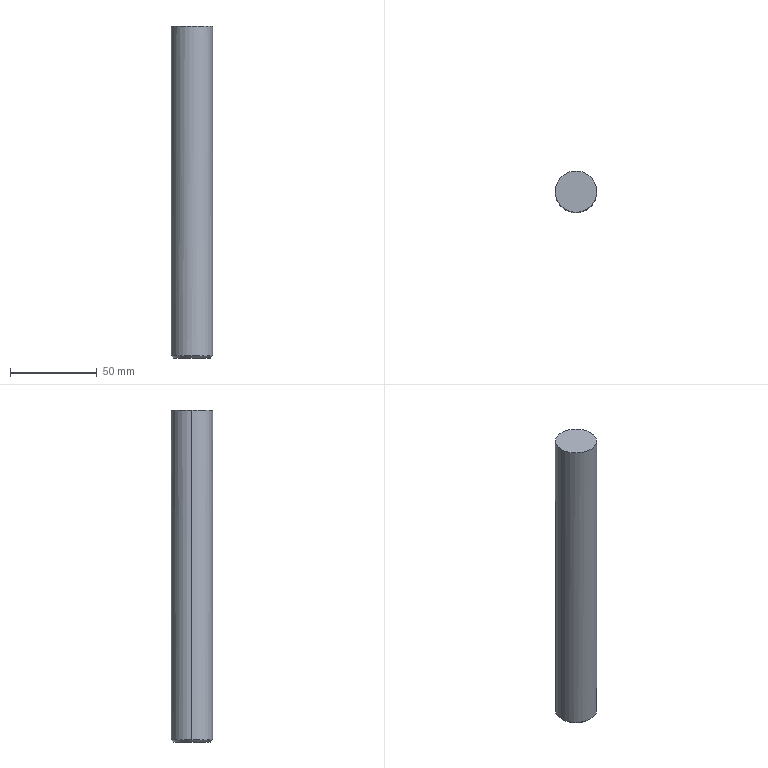Part | SolidWorks | features BaseBody 1 | 1 solid | 13 faces | box 23.8 x 23.8 x 191 mm | volume 54008 mm3 | plane 6 | cylinder 5 | cone 2 | commonest cylinder face diameters 14 x3 23.8 x2
STEP:
#1=CARTESIAN_POINT('',(0.,11.9,-103.8));
#2=VERTEX_POINT('',#1);
#3=CARTESIAN_POINT('',(-11.9,0.,-103.8));
#4=VERTEX_POINT('',#3);
#5=CARTESIAN_POINT('',(0.,0.,-103.8));
#6=DIRECTION('',(0.,0.,1.));
#7=DIRECTION('',(1.,0.,0.));
#8=AXIS2_PLACEMENT_3D('',#5,#6,#7);
#9=CIRCLE('',#8,11.9);
#10=EDGE_CURVE('',#2,#4,#9,.T.);
#11=ORIENTED_EDGE('',*,*,#10,.T.);
#12=CARTESIAN_POINT('',(-11.9,0.,86.));
#13=VERTEX_POINT('',#12);
#14=CARTESIAN_POINT('',(-11.9,0.,90.));
#15=DIRECTION('',(0.,0.,1.));
#16=VECTOR('',#15,1000.);
#17=LINE('',#14,#16);
#18=EDGE_CURVE('',#4,#13,#17,.T.);
#19=ORIENTED_EDGE('',*,*,#18,.T.);
#20=CARTESIAN_POINT('',(11.9,0.,86.));
#21=VERTEX_POINT('',#20);
#22=CARTESIAN_POINT('',(0.,0.,86.));
#23=DIRECTION('',(0.,0.,-1.));
#24=DIRECTION('',(1.,0.,0.));
#25=AXIS2_PLACEMENT_3D('',#22,#23,#24);
#26=CIRCLE('',#25,11.9);
#27=EDGE_CURVE('',#13,#21,#26,.T.);
#28=ORIENTED_EDGE('',*,*,#27,.T.);
#29=CARTESIAN_POINT('',(11.9,0.,-103.8));
#30=VERTEX_POINT('',#29);
#31=CARTESIAN_POINT('',(11.9,0.,90.));
#32=DIRECTION('',(0.,0.,1.));
#33=VECTOR('',#32,1000.);
#34=LINE('',#31,#33);
#35=EDGE_CURVE('',#30,#21,#34,.T.);
#36=ORIENTED_EDGE('',*,*,#35,.F.);
#37=CARTESIAN_POINT('',(0.,0.,-103.8));
#38=DIRECTION('',(0.,0.,1.));
#39=DIRECTION('',(1.,0.,0.));
#40=AXIS2_PLACEMENT_3D('',#37,#38,#39);
#41=CIRCLE('',#40,11.9);
#42=EDGE_CURVE('',#30,#2,#41,.T.);
#43=ORIENTED_EDGE('',*,*,#42,.T.);
#44=EDGE_LOOP('',(#11,#19,#28,#36,#43));
#45=FACE_OUTER_BOUND('',#44,.T.);
#46=CARTESIAN_POINT('',(0.,0.,90.));
#47=DIRECTION('',(0.,0.,1.));
#48=DIRECTION('',(1.,0.,0.));
#49=AXIS2_PLACEMENT_3D('',#46,#47,#48);
#50=CYLINDRICAL_SURFACE('',#49,11.9);
#51=ADVANCED_FACE('',(#45),#50,.T.);
#52=CARTESIAN_POINT('',(0.,-10.7,-105.));
#53=VERTEX_POINT('',#52);
#54=CARTESIAN_POINT('',(0.,10.7,-105.));
#55=VERTEX_POINT('',#54);
#56=CARTESIAN_POINT('',(0.,0.,-105.));
#57=DIRECTION('',(0.,0.,1.));
#58=DIRECTION('',(0.,-1.,0.));
#59=AXIS2_PLACEMENT_3D('',#56,#57,#58);
#60=CIRCLE('',#59,10.7);
#61=EDGE_CURVE('',#53,#55,#60,.T.);
#62=ORIENTED_EDGE('',*,*,#61,.T.);
#63=CARTESIAN_POINT('',(0.,11.9,-103.8));
#64=DIRECTION('',(0.,0.7071,0.7071));
#65=VECTOR('',#64,1000.);
#66=LINE('',#63,#65);
#67=EDGE_CURVE('',#55,#2,#66,.T.);
#68=ORIENTED_EDGE('',*,*,#67,.T.);
#69=ORIENTED_EDGE('',*,*,#42,.F.);
#70=CARTESIAN_POINT('',(0.,-11.9,-103.8));
#71=VERTEX_POINT('',#70);
#72=CARTESIAN_POINT('',(0.,0.,-103.8));
#73=DIRECTION('',(0.,0.,1.));
#74=DIRECTION('',(1.,0.,0.));
#75=AXIS2_PLACEMENT_3D('',#72,#73,#74);
#76=CIRCLE('',#75,11.9);
#77=EDGE_CURVE('',#71,#30,#76,.T.);
#78=ORIENTED_EDGE('',*,*,#77,.F.);
#79=CARTESIAN_POINT('',(0.,-11.9,-103.8));
#80=DIRECTION('',(0.,-0.7071,0.7071));
#81=VECTOR('',#80,1000.);
#82=LINE('',#79,#81);
#83=EDGE_CURVE('',#53,#71,#82,.T.);
#84=ORIENTED_EDGE('',*,*,#83,.F.);
#85=EDGE_LOOP('',(#62,#68,#69,#78,#84));
#86=FACE_OUTER_BOUND('',#85,.T.);
#87=CARTESIAN_POINT('',(0.,0.,-103.8));
#88=DIRECTION('',(0.,0.,1.));
#89=DIRECTION('',(0.,-1.,0.));
#90=AXIS2_PLACEMENT_3D('',#87,#88,#89);
#91=CONICAL_SURFACE('',#90,11.9,0.7854);
#92=ADVANCED_FACE('',(#86),#91,.T.);
#93=CARTESIAN_POINT('',(7.,0.,-105.));
#94=VERTEX_POINT('',#93);
#95=CARTESIAN_POINT('',(-7.,0.,-105.));
#96=VERTEX_POINT('',#95);
#97=CARTESIAN_POINT('',(0.,0.,-105.));
#98=DIRECTION('',(0.,0.,-1.));
#99=DIRECTION('',(1.,0.,0.));
#100=AXIS2_PLACEMENT_3D('',#97,#98,#99);
#101=CIRCLE('',#100,7.);
#102=EDGE_CURVE('',#94,#96,#101,.T.);
#103=ORIENTED_EDGE('',*,*,#102,.T.);
#104=CARTESIAN_POINT('',(-7.,0.,81.));
#105=VERTEX_POINT('',#104);
#106=CARTESIAN_POINT('',(-7.,0.,90.));
#107=DIRECTION('',(0.,0.,1.));
#108=VECTOR('',#107,1000.);
#109=LINE('',#106,#108);
#110=EDGE_CURVE('',#96,#105,#109,.T.);
#111=ORIENTED_EDGE('',*,*,#110,.T.);
#112=CARTESIAN_POINT('',(7.,0.,81.));
#113=VERTEX_POINT('',#112);
#114=CARTESIAN_POINT('',(0.,0.,81.));
#115=DIRECTION('',(0.,0.,-1.));
#116=DIRECTION('',(1.,0.,0.));
#117=AXIS2_PLACEMENT_3D('',#114,#115,#116);
#118=CIRCLE('',#117,7.);
#119=EDGE_CURVE('',#113,#105,#118,.T.);
#120=ORIENTED_EDGE('',*,*,#119,.F.);
#121=CARTESIAN_POINT('',(7.,0.,90.));
#122=DIRECTION('',(0.,0.,1.));
#123=VECTOR('',#122,1000.);
#124=LINE('',#121,#123);
#125=EDGE_CURVE('',#94,#113,#124,.T.);
#126=ORIENTED_EDGE('',*,*,#125,.F.);
#127=EDGE_LOOP('',(#103,#111,#120,#126));
#128=FACE_OUTER_BOUND('',#127,.T.);
#129=CARTESIAN_POINT('',(0.,0.,90.));
#130=DIRECTION('',(0.,0.,1.));
#131=DIRECTION('',(1.,0.,0.));
#132=AXIS2_PLACEMENT_3D('',#129,#130,#131);
#133=CYLINDRICAL_SURFACE('',#132,7.);
#134=ADVANCED_FACE('',(#128),#133,.F.);
#135=CARTESIAN_POINT('',(2.5,6.538,-105.));
#136=VERTEX_POINT('',#135);
#137=CARTESIAN_POINT('',(0.,0.,-105.));
#138=DIRECTION('',(0.,0.,-1.));
#139=DIRECTION('',(1.,0.,0.));
#140=AXIS2_PLACEMENT_3D('',#137,#138,#139);
#141=CIRCLE('',#140,7.);
#142=EDGE_CURVE('',#136,#94,#141,.T.);
#143=ORIENTED_EDGE('',*,*,#142,.T.);
#144=ORIENTED_EDGE('',*,*,#125,.T.);
#145=CARTESIAN_POINT('',(2.5,6.538,81.));
#146=VERTEX_POINT('',#145);
#147=CARTESIAN_POINT('',(0.,0.,81.));
#148=DIRECTION('',(0.,0.,-1.));
#149=DIRECTION('',(1.,0.,0.));
#150=AXIS2_PLACEMENT_3D('',#147,#148,#149);
#151=CIRCLE('',#150,7.);
#152=EDGE_CURVE('',#146,#113,#151,.T.);
#153=ORIENTED_EDGE('',*,*,#152,.F.);
#154=CARTESIAN_POINT('',(2.5,6.538,90.));
#155=DIRECTION('',(0.,0.,1.));
#156=VECTOR('',#155,1000.);
#157=LINE('',#154,#156);
#158=EDGE_CURVE('',#136,#146,#157,.T.);
#159=ORIENTED_EDGE('',*,*,#158,.F.);
#160=EDGE_LOOP('',(#143,#144,#153,#159));
#161=FACE_OUTER_BOUND('',#160,.T.);
#162=CARTESIAN_POINT('',(0.,0.,90.));
#163=DIRECTION('',(0.,0.,1.));
#164=DIRECTION('',(1.,0.,0.));
#165=AXIS2_PLACEMENT_3D('',#162,#163,#164);
#166=CYLINDRICAL_SURFACE('',#165,7.);
#167=ADVANCED_FACE('',(#161),#166,.F.);
#168=ORIENTED_EDGE('',*,*,#18,.F.);
#169=CARTESIAN_POINT('',(0.,0.,-103.8));
#170=DIRECTION('',(0.,0.,1.));
#171=DIRECTION('',(1.,0.,0.));
#172=AXIS2_PLACEMENT_3D('',#169,#170,#171);
#173=CIRCLE('',#172,11.9);
#174=EDGE_CURVE('',#4,#71,#173,.T.);
#175=ORIENTED_EDGE('',*,*,#174,.T.);
#176=ORIENTED_EDGE('',*,*,#77,.T.);
#177=ORIENTED_EDGE('',*,*,#35,.T.);
#178=CARTESIAN_POINT('',(0.,0.,86.));
#179=DIRECTION('',(0.,0.,-1.));
#180=DIRECTION('',(1.,0.,0.));
#181=AXIS2_PLACEMENT_3D('',#178,#179,#180);
#182=CIRCLE('',#181,11.9);
#183=EDGE_CURVE('',#21,#13,#182,.T.);
#184=ORIENTED_EDGE('',*,*,#183,.T.);
#185=EDGE_LOOP('',(#168,#175,#176,#177,#184));
#186=FACE_OUTER_BOUND('',#185,.T.);
#187=CARTESIAN_POINT('',(0.,0.,90.));
#188=DIRECTION('',(0.,0.,1.));
#189=DIRECTION('',(1.,0.,0.));
#190=AXIS2_PLACEMENT_3D('',#187,#188,#189);
#191=CYLINDRICAL_SURFACE('',#190,11.9);
#192=ADVANCED_FACE('',(#186),#191,.T.);
#193=ORIENTED_EDGE('',*,*,#183,.F.);
#194=ORIENTED_EDGE('',*,*,#27,.F.);
#195=EDGE_LOOP('',(#193,#194));
#196=FACE_OUTER_BOUND('',#195,.T.);
#197=CARTESIAN_POINT('',(0.,11.9,86.));
#198=DIRECTION('',(0.,0.,-1.));
#199=DIRECTION('',(-1.,0.,0.));
#200=AXIS2_PLACEMENT_3D('',#197,#198,#199);
#201=PLANE('',#200);
#202=ADVANCED_FACE('',(#196),#201,.F.);
#203=ORIENTED_EDGE('',*,*,#67,.F.);
#204=CARTESIAN_POINT('',(0.,0.,-105.));
#205=DIRECTION('',(0.,0.,1.));
#206=DIRECTION('',(0.,-1.,0.));
#207=AXIS2_PLACEMENT_3D('',#204,#205,#206);
#208=CIRCLE('',#207,10.7);
#209=EDGE_CURVE('',#55,#53,#208,.T.);
#210=ORIENTED_EDGE('',*,*,#209,.T.);
#211=ORIENTED_EDGE('',*,*,#83,.T.);
#212=ORIENTED_EDGE('',*,*,#174,.F.);
#213=ORIENTED_EDGE('',*,*,#10,.F.);
#214=EDGE_LOOP('',(#203,#210,#211,#212,#213));
#215=FACE_OUTER_BOUND('',#214,.T.);
#216=CARTESIAN_POINT('',(0.,0.,-103.8));
#217=DIRECTION('',(0.,0.,1.));
#218=DIRECTION('',(0.,-1.,0.));
#219=AXIS2_PLACEMENT_3D('',#216,#217,#218);
#220=CONICAL_SURFACE('',#219,11.9,0.7854);
#221=ADVANCED_FACE('',(#215),#220,.T.);
#222=ORIENTED_EDGE('',*,*,#142,.F.);
#223=CARTESIAN_POINT('',(2.5,9.3,-105.));
#224=VERTEX_POINT('',#223);
#225=CARTESIAN_POINT('',(2.5,7.,-105.));
#226=DIRECTION('',(0.,-1.,0.));
#227=VECTOR('',#226,1000.);
#228=LINE('',#225,#227);
#229=EDGE_CURVE('',#224,#136,#228,.T.);
#230=ORIENTED_EDGE('',*,*,#229,.F.);
#231=CARTESIAN_POINT('',(-2.5,9.3,-105.));
#232=VERTEX_POINT('',#231);
#233=CARTESIAN_POINT('',(0.,9.3,-105.));
#234=DIRECTION('',(1.,0.,0.));
#235=VECTOR('',#234,1000.);
#236=LINE('',#233,#235);
#237=EDGE_CURVE('',#232,#224,#236,.T.);
#238=ORIENTED_EDGE('',*,*,#237,.F.);
#239=CARTESIAN_POINT('',(-2.5,6.538,-105.));
#240=VERTEX_POINT('',#239);
#241=CARTESIAN_POINT('',(-2.5,7.,-105.));
#242=DIRECTION('',(0.,1.,0.));
#243=VECTOR('',#242,1000.);
#244=LINE('',#241,#243);
#245=EDGE_CURVE('',#240,#232,#244,.T.);
#246=ORIENTED_EDGE('',*,*,#245,.F.);
#247=CARTESIAN_POINT('',(0.,0.,-105.));
#248=DIRECTION('',(0.,0.,-1.));
#249=DIRECTION('',(1.,0.,0.));
#250=AXIS2_PLACEMENT_3D('',#247,#248,#249);
#251=CIRCLE('',#250,7.);
#252=EDGE_CURVE('',#96,#240,#251,.T.);
#253=ORIENTED_EDGE('',*,*,#252,.F.);
#254=ORIENTED_EDGE('',*,*,#102,.F.);
#255=EDGE_LOOP('',(#222,#230,#238,#246,#253,#254));
#256=FACE_BOUND('',#255,.T.);
#257=ORIENTED_EDGE('',*,*,#61,.F.);
#258=ORIENTED_EDGE('',*,*,#209,.F.);
#259=EDGE_LOOP('',(#257,#258));
#260=FACE_OUTER_BOUND('',#259,.T.);
#261=CARTESIAN_POINT('',(0.,7.,-105.));
#262=DIRECTION('',(0.,0.,1.));
#263=DIRECTION('',(1.,0.,0.));
#264=AXIS2_PLACEMENT_3D('',#261,#262,#263);
#265=PLANE('',#264);
#266=ADVANCED_FACE('',(#256,#260),#265,.F.);
#267=ORIENTED_EDGE('',*,*,#110,.F.);
#268=ORIENTED_EDGE('',*,*,#252,.T.);
#269=CARTESIAN_POINT('',(-2.5,6.538,81.));
#270=VERTEX_POINT('',#269);
#271=CARTESIAN_POINT('',(-2.5,6.538,90.));
#272=DIRECTION('',(0.,0.,-1.));
#273=VECTOR('',#272,1000.);
#274=LINE('',#271,#273);
#275=EDGE_CURVE('',#270,#240,#274,.T.);
#276=ORIENTED_EDGE('',*,*,#275,.F.);
#277=CARTESIAN_POINT('',(0.,0.,81.));
#278=DIRECTION('',(0.,0.,-1.));
#279=DIRECTION('',(1.,0.,0.));
#280=AXIS2_PLACEMENT_3D('',#277,#278,#279);
#281=CIRCLE('',#280,7.);
#282=EDGE_CURVE('',#105,#270,#281,.T.);
#283=ORIENTED_EDGE('',*,*,#282,.F.);
#284=EDGE_LOOP('',(#267,#268,#276,#283));
#285=FACE_OUTER_BOUND('',#284,.T.);
#286=CARTESIAN_POINT('',(0.,0.,90.));
#287=DIRECTION('',(0.,0.,1.));
#288=DIRECTION('',(1.,0.,0.));
#289=AXIS2_PLACEMENT_3D('',#286,#287,#288);
#290=CYLINDRICAL_SURFACE('',#289,7.);
#291=ADVANCED_FACE('',(#285),#290,.F.);
#292=ORIENTED_EDGE('',*,*,#229,.T.);
#293=ORIENTED_EDGE('',*,*,#158,.T.);
#294=CARTESIAN_POINT('',(2.5,9.3,81.));
#295=VERTEX_POINT('',#294);
#296=CARTESIAN_POINT('',(2.5,9.3,81.));
#297=DIRECTION('',(0.,-1.,0.));
#298=VECTOR('',#297,1000.);
#299=LINE('',#296,#298);
#300=EDGE_CURVE('',#295,#146,#299,.T.);
#301=ORIENTED_EDGE('',*,*,#300,.F.);
#302=CARTESIAN_POINT('',(2.5,9.3,-105.));
#303=DIRECTION('',(0.,0.,1.));
#304=VECTOR('',#303,1000.);
#305=LINE('',#302,#304);
#306=EDGE_CURVE('',#224,#295,#305,.T.);
#307=ORIENTED_EDGE('',*,*,#306,.F.);
#308=EDGE_LOOP('',(#292,#293,#301,#307));
#309=FACE_OUTER_BOUND('',#308,.T.);
#310=CARTESIAN_POINT('',(2.5,9.3,-105.));
#311=DIRECTION('',(1.,0.,0.));
#312=DIRECTION('',(0.,1.,0.));
#313=AXIS2_PLACEMENT_3D('',#310,#311,#312);
#314=PLANE('',#313);
#315=ADVANCED_FACE('',(#309),#314,.F.);
#316=ORIENTED_EDGE('',*,*,#237,.T.);
#317=ORIENTED_EDGE('',*,*,#306,.T.);
#318=CARTESIAN_POINT('',(-2.5,9.3,81.));
#319=VERTEX_POINT('',#318);
#320=CARTESIAN_POINT('',(-2.5,9.3,81.));
#321=DIRECTION('',(1.,0.,0.));
#322=VECTOR('',#321,1000.);
#323=LINE('',#320,#322);
#324=EDGE_CURVE('',#319,#295,#323,.T.);
#325=ORIENTED_EDGE('',*,*,#324,.F.);
#326=CARTESIAN_POINT('',(-2.5,9.3,-105.));
#327=DIRECTION('',(0.,0.,1.));
#328=VECTOR('',#327,1000.);
#329=LINE('',#326,#328);
#330=EDGE_CURVE('',#232,#319,#329,.T.);
#331=ORIENTED_EDGE('',*,*,#330,.F.);
#332=EDGE_LOOP('',(#316,#317,#325,#331));
#333=FACE_OUTER_BOUND('',#332,.T.);
#334=CARTESIAN_POINT('',(-2.5,9.3,-105.));
#335=DIRECTION('',(0.,1.,0.));
#336=DIRECTION('',(0.,0.,1.));
#337=AXIS2_PLACEMENT_3D('',#334,#335,#336);
#338=PLANE('',#337);
#339=ADVANCED_FACE('',(#333),#338,.F.);
#340=ORIENTED_EDGE('',*,*,#245,.T.);
#341=ORIENTED_EDGE('',*,*,#330,.T.);
#342=CARTESIAN_POINT('',(-2.5,6.538,81.));
#343=DIRECTION('',(0.,1.,0.));
#344=VECTOR('',#343,1000.);
#345=LINE('',#342,#344);
#346=EDGE_CURVE('',#270,#319,#345,.T.);
#347=ORIENTED_EDGE('',*,*,#346,.F.);
#348=ORIENTED_EDGE('',*,*,#275,.T.);
#349=EDGE_LOOP('',(#340,#341,#347,#348));
#350=FACE_OUTER_BOUND('',#349,.T.);
#351=CARTESIAN_POINT('',(-2.5,6.538,-105.));
#352=DIRECTION('',(-1.,0.,0.));
#353=DIRECTION('',(0.,-1.,0.));
#354=AXIS2_PLACEMENT_3D('',#351,#352,#353);
#355=PLANE('',#354);
#356=ADVANCED_FACE('',(#350),#355,.F.);
#357=ORIENTED_EDGE('',*,*,#346,.T.);
#358=ORIENTED_EDGE('',*,*,#324,.T.);
#359=ORIENTED_EDGE('',*,*,#300,.T.);
#360=ORIENTED_EDGE('',*,*,#152,.T.);
#361=ORIENTED_EDGE('',*,*,#119,.T.);
#362=ORIENTED_EDGE('',*,*,#282,.T.);
#363=EDGE_LOOP('',(#357,#358,#359,#360,#361,#362));
#364=FACE_OUTER_BOUND('',#363,.T.);
#365=CARTESIAN_POINT('',(0.,7.,81.));
#366=DIRECTION('',(0.,0.,1.));
#367=DIRECTION('',(1.,0.,0.));
#368=AXIS2_PLACEMENT_3D('',#365,#366,#367);
#369=PLANE('',#368);
#370=ADVANCED_FACE('',(#364),#369,.F.);
#371=CLOSED_SHELL('',(#51,#92,#134,#167,#192,#202,#221,#266,#291,#315,#339,#356,#370));
#372=MANIFOLD_SOLID_BREP('',#371);
#373=CARTESIAN_POINT('',(0.,0.,0.));
#374=DIRECTION('',(0.,0.,1.));
#375=DIRECTION('',(1.,0.,0.));
#376=AXIS2_PLACEMENT_3D('',#373,#374,#375);
#377=(LENGTH_UNIT()NAMED_UNIT(*)SI_UNIT(.MILLI.,.METRE.));
#378=UNCERTAINTY_MEASURE_WITH_UNIT(LENGTH_MEASURE(0.00001),#377,'','');
#379=(NAMED_UNIT(*)PLANE_ANGLE_UNIT()SI_UNIT($,.RADIAN.));
#380=(NAMED_UNIT(*)SI_UNIT($,.STERADIAN.)SOLID_ANGLE_UNIT());
#381=(GEOMETRIC_REPRESENTATION_CONTEXT(3)GLOBAL_UNCERTAINTY_ASSIGNED_CONTEXT((#378))GLOBAL_UNIT_ASSIGNED_CONTEXT((#377,#379,#380))REPRESENTATION_CONTEXT('',''));
#382=ADVANCED_BREP_SHAPE_REPRESENTATION('',(#372,#376),#381);